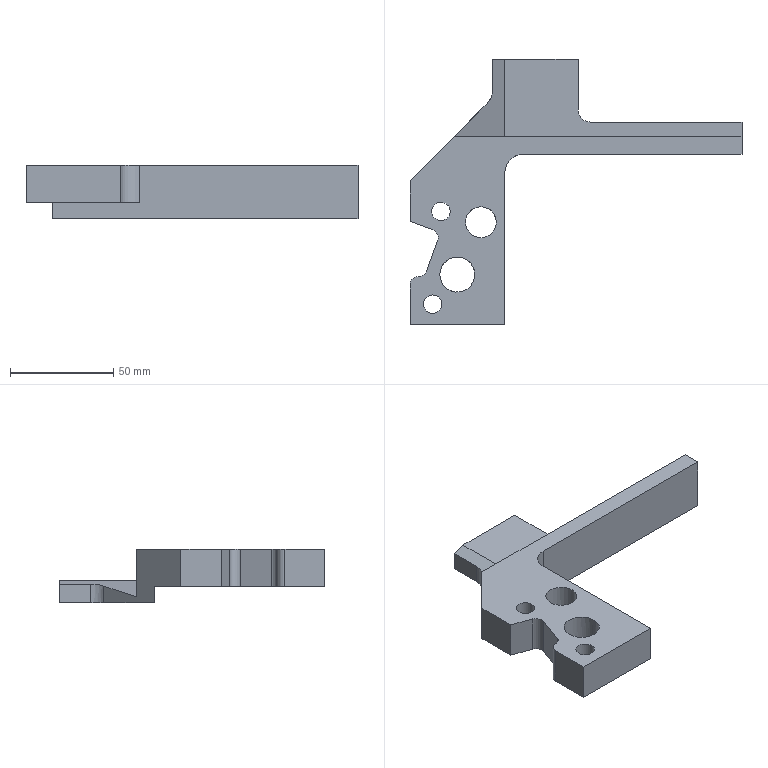Part | STEP file | gslz 2016.10.28-13_id786_x_t | 1 solid | 33 faces | box 161 x 128.857 x 26 mm | volume 106993 mm3 | plane 21 | cylinder 12 | commonest cylinder face diameters 8 x3 15 x3 9 x2 18 x2 12 x1 17 x1